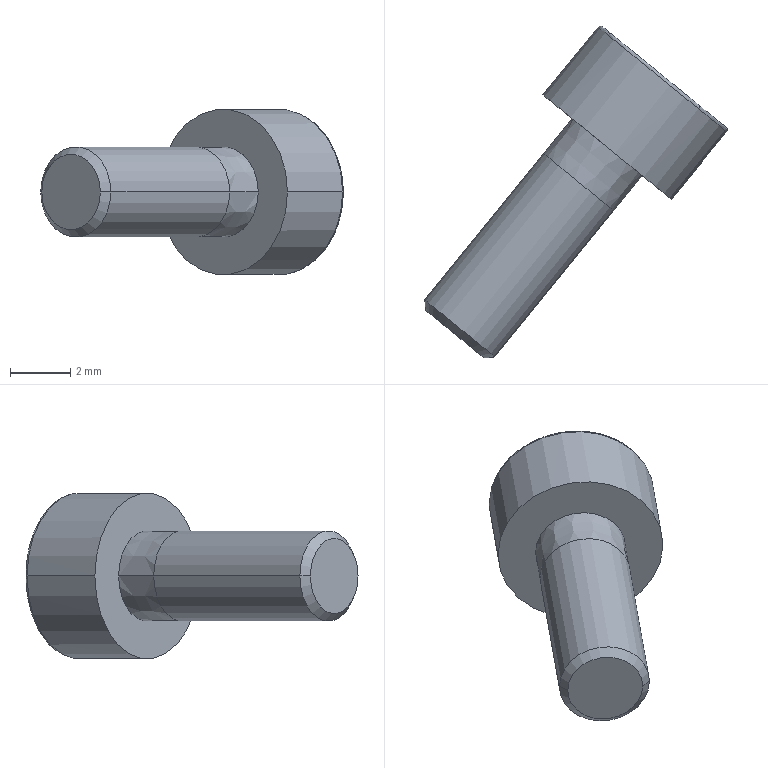Part | SolidWorks | features BaseBody 1 | 1 solid | 20 faces | box 10.039 x 11.017 x 5.5 mm | volume 120.466 mm3 | plane 10 | cylinder 4 | cone 4 | spline 2 | commonest cylinder face diameters 3 x2 5.5 x2
STEP:
#1=CARTESIAN_POINT('',(545.105,-162.622,308.898));
#2=VERTEX_POINT('',#1);
#3=CARTESIAN_POINT('',(541.772,-159.912,306.624));
#4=VERTEX_POINT('',#3);
#5=CARTESIAN_POINT('',(543.905,-161.647,306.624));
#6=DIRECTION('',(-0.6309,-0.7758,0.000000012));
#7=DIRECTION('',(0.7758,-0.6309,0.));
#8=AXIS2_PLACEMENT_3D('',#5,#6,#7);
#9=CIRCLE('',#8,2.75);
#10=EDGE_CURVE('',#2,#4,#9,.T.);
#11=ORIENTED_EDGE('',*,*,#10,.F.);
#12=CARTESIAN_POINT('',(545.124,-162.509,308.815));
#13=VERTEX_POINT('',#12);
#14=CARTESIAN_POINT('',(545.061,-162.587,308.815));
#15=DIRECTION('',(-0.6417,0.5218,0.5621));
#16=DIRECTION('',(0.4361,-0.3546,0.8271));
#17=AXIS2_PLACEMENT_3D('',#14,#15,#16);
#18=CIRCLE('',#17,0.1);
#19=EDGE_CURVE('',#2,#13,#18,.T.);
#20=ORIENTED_EDGE('',*,*,#19,.T.);
#21=CARTESIAN_POINT('',(542.813,-160.63,304.432));
#22=VERTEX_POINT('',#21);
#23=CARTESIAN_POINT('',(545.124,-162.509,308.815));
#24=CARTESIAN_POINT('',(541.723,-159.744,311.794));
#25=CARTESIAN_POINT('',(539.412,-157.864,307.411));
#26=CARTESIAN_POINT('',(542.813,-160.63,304.432));
#27=(BOUNDED_CURVE()B_SPLINE_CURVE(3,(#23,#24,#25,#26),.UNSPECIFIED.,.F.,.F.)B_SPLINE_CURVE_WITH_KNOTS((4,4),(0.,1.),.UNSPECIFIED.)CURVE()GEOMETRIC_REPRESENTATION_ITEM()RATIONAL_B_SPLINE_CURVE((1.,0.3333,0.3333,1.))REPRESENTATION_ITEM(''));
#28=EDGE_CURVE('',#13,#22,#27,.T.);
#29=ORIENTED_EDGE('',*,*,#28,.T.);
#30=CARTESIAN_POINT('',(542.706,-160.672,304.349));
#31=VERTEX_POINT('',#30);
#32=CARTESIAN_POINT('',(542.75,-160.707,304.432));
#33=DIRECTION('',(0.6417,-0.5218,-0.5621));
#34=DIRECTION('',(-0.4361,0.3546,-0.8271));
#35=AXIS2_PLACEMENT_3D('',#32,#33,#34);
#36=CIRCLE('',#35,0.1);
#37=EDGE_CURVE('',#31,#22,#36,.T.);
#38=ORIENTED_EDGE('',*,*,#37,.F.);
#39=CARTESIAN_POINT('',(543.905,-161.647,306.624));
#40=DIRECTION('',(-0.6309,-0.7758,0.000000012));
#41=DIRECTION('',(0.7758,-0.6309,0.));
#42=AXIS2_PLACEMENT_3D('',#39,#40,#41);
#43=CIRCLE('',#42,2.75);
#44=EDGE_CURVE('',#4,#31,#43,.T.);
#45=ORIENTED_EDGE('',*,*,#44,.F.);
#46=EDGE_LOOP('',(#11,#20,#29,#38,#45));
#47=FACE_OUTER_BOUND('',#46,.T.);
#48=CARTESIAN_POINT('',(545.105,-162.622,308.898));
#49=CARTESIAN_POINT('',(541.575,-159.752,311.99));
#50=CARTESIAN_POINT('',(539.177,-157.802,307.441));
#51=CARTESIAN_POINT('',(542.706,-160.672,304.349));
#52=CARTESIAN_POINT('',(545.142,-162.577,308.898));
#53=CARTESIAN_POINT('',(541.612,-159.707,311.99));
#54=CARTESIAN_POINT('',(539.214,-157.756,307.441));
#55=CARTESIAN_POINT('',(542.743,-160.627,304.349));
#56=CARTESIAN_POINT('',(545.15,-162.53,308.864));
#57=CARTESIAN_POINT('',(541.674,-159.703,311.909));
#58=CARTESIAN_POINT('',(539.311,-157.782,307.428));
#59=CARTESIAN_POINT('',(542.787,-160.609,304.383));
#60=CARTESIAN_POINT('',(545.124,-162.509,308.815));
#61=CARTESIAN_POINT('',(541.723,-159.744,311.794));
#62=CARTESIAN_POINT('',(539.412,-157.864,307.411));
#63=CARTESIAN_POINT('',(542.813,-160.63,304.432));
#64=(BOUNDED_SURFACE()B_SPLINE_SURFACE(3,3,((#48,#49,#50,#51),(#52,#53,#54,#55),(#56,#57,#58,#59),(#60,#61,#62,#63)),.UNSPECIFIED.,.F.,.F.,.F.)B_SPLINE_SURFACE_WITH_KNOTS((4,4),(4,4),(0.,1.),(0.,1.),.UNSPECIFIED.)GEOMETRIC_REPRESENTATION_ITEM()RATIONAL_B_SPLINE_SURFACE(((1.,0.3333,0.3333,1.),(0.8047,0.2682,0.2682,0.8047),(0.8047,0.2682,0.2682,0.8047),(1.,0.3333,0.3333,1.)))REPRESENTATION_ITEM('')SURFACE());
#65=ADVANCED_FACE('',(#47),#64,.T.);
#66=CARTESIAN_POINT('',(542.293,-166.007,306.624));
#67=VERTEX_POINT('',#66);
#68=CARTESIAN_POINT('',(539.966,-164.115,306.624));
#69=VERTEX_POINT('',#68);
#70=CARTESIAN_POINT('',(541.129,-165.061,306.624));
#71=DIRECTION('',(-0.6309,-0.7758,0.000000012));
#72=DIRECTION('',(0.7758,-0.6309,0.));
#73=AXIS2_PLACEMENT_3D('',#70,#71,#72);
#74=CIRCLE('',#73,1.5);
#75=EDGE_CURVE('',#67,#69,#74,.T.);
#76=ORIENTED_EDGE('',*,*,#75,.T.);
#77=CARTESIAN_POINT('',(536.022,-168.964,306.624));
#78=VERTEX_POINT('',#77);
#79=CARTESIAN_POINT('',(537.994,-166.539,306.624));
#80=DIRECTION('',(-0.6309,-0.7758,0.000000012));
#81=VECTOR('',#80,1000.);
#82=LINE('',#79,#81);
#83=EDGE_CURVE('',#69,#78,#82,.T.);
#84=ORIENTED_EDGE('',*,*,#83,.T.);
#85=CARTESIAN_POINT('',(538.35,-170.856,306.624));
#86=VERTEX_POINT('',#85);
#87=CARTESIAN_POINT('',(537.186,-169.91,306.624));
#88=DIRECTION('',(0.6309,0.7758,-0.000000012));
#89=DIRECTION('',(0.7758,-0.6309,0.));
#90=AXIS2_PLACEMENT_3D('',#87,#88,#89);
#91=CIRCLE('',#90,1.5);
#92=EDGE_CURVE('',#78,#86,#91,.T.);
#93=ORIENTED_EDGE('',*,*,#92,.T.);
#94=CARTESIAN_POINT('',(540.321,-168.432,306.624));
#95=DIRECTION('',(-0.6309,-0.7758,0.000000012));
#96=VECTOR('',#95,1000.);
#97=LINE('',#94,#96);
#98=EDGE_CURVE('',#67,#86,#97,.T.);
#99=ORIENTED_EDGE('',*,*,#98,.F.);
#100=EDGE_LOOP('',(#76,#84,#93,#99));
#101=FACE_OUTER_BOUND('',#100,.T.);
#102=CARTESIAN_POINT('',(539.158,-167.485,306.624));
#103=DIRECTION('',(-0.6309,-0.7758,0.000000012));
#104=DIRECTION('',(0.7758,-0.6309,0.));
#105=AXIS2_PLACEMENT_3D('',#102,#103,#104);
#106=CYLINDRICAL_SURFACE('',#105,1.5);
#107=ADVANCED_FACE('',(#101),#106,.T.);
#108=CARTESIAN_POINT('',(543.239,-164.843,306.624));
#109=VERTEX_POINT('',#108);
#110=CARTESIAN_POINT('',(540.913,-162.951,306.624));
#111=VERTEX_POINT('',#110);
#112=CARTESIAN_POINT('',(542.076,-163.897,306.624));
#113=DIRECTION('',(-0.6309,-0.7758,0.000000012));
#114=DIRECTION('',(0.7758,-0.6309,0.));
#115=AXIS2_PLACEMENT_3D('',#112,#113,#114);
#116=CIRCLE('',#115,1.499);
#117=EDGE_CURVE('',#109,#111,#116,.T.);
#118=ORIENTED_EDGE('',*,*,#117,.T.);
#119=CARTESIAN_POINT('',(539.966,-164.115,306.624));
#120=DIRECTION('',(-0.6313,-0.7755,0.000000012));
#121=VECTOR('',#120,1000.);
#122=LINE('',#119,#121);
#123=EDGE_CURVE('',#111,#69,#122,.T.);
#124=ORIENTED_EDGE('',*,*,#123,.T.);
#125=ORIENTED_EDGE('',*,*,#75,.F.);
#126=CARTESIAN_POINT('',(542.293,-166.007,306.624));
#127=DIRECTION('',(-0.6305,-0.7762,0.000000012));
#128=VECTOR('',#127,1000.);
#129=LINE('',#126,#128);
#130=EDGE_CURVE('',#109,#67,#129,.T.);
#131=ORIENTED_EDGE('',*,*,#130,.F.);
#132=EDGE_LOOP('',(#118,#124,#125,#131));
#133=FACE_OUTER_BOUND('',#132,.T.);
#134=CARTESIAN_POINT('',(541.129,-165.061,306.624));
#135=DIRECTION('',(-0.6309,-0.7758,0.000000012));
#136=DIRECTION('',(0.7758,-0.6309,0.));
#137=AXIS2_PLACEMENT_3D('',#134,#135,#136);
#138=CONICAL_SURFACE('',#137,1.5,0.0005);
#139=ADVANCED_FACE('',(#133),#138,.T.);
#140=CARTESIAN_POINT('',(536.058,-169.315,306.624));
#141=VERTEX_POINT('',#140);
#142=CARTESIAN_POINT('',(537.998,-170.893,306.624));
#143=VERTEX_POINT('',#142);
#144=CARTESIAN_POINT('',(537.028,-170.104,306.624));
#145=DIRECTION('',(0.6309,0.7758,-0.000000012));
#146=DIRECTION('',(-0.7758,0.6309,0.));
#147=AXIS2_PLACEMENT_3D('',#144,#145,#146);
#148=CIRCLE('',#147,1.25);
#149=EDGE_CURVE('',#141,#143,#148,.T.);
#150=ORIENTED_EDGE('',*,*,#149,.T.);
#151=CARTESIAN_POINT('',(538.35,-170.856,306.624));
#152=DIRECTION('',(0.9947,0.1025,-0.000000009));
#153=VECTOR('',#152,1000.);
#154=LINE('',#151,#153);
#155=EDGE_CURVE('',#143,#86,#154,.T.);
#156=ORIENTED_EDGE('',*,*,#155,.T.);
#157=ORIENTED_EDGE('',*,*,#92,.F.);
#158=CARTESIAN_POINT('',(536.022,-168.964,306.624));
#159=DIRECTION('',(-0.1025,0.9947,-0.000000009));
#160=VECTOR('',#159,1000.);
#161=LINE('',#158,#160);
#162=EDGE_CURVE('',#141,#78,#161,.T.);
#163=ORIENTED_EDGE('',*,*,#162,.F.);
#164=EDGE_LOOP('',(#150,#156,#157,#163));
#165=FACE_OUTER_BOUND('',#164,.T.);
#166=CARTESIAN_POINT('',(537.186,-169.91,306.624));
#167=DIRECTION('',(0.6309,0.7758,-0.000000012));
#168=DIRECTION('',(-0.7758,0.6309,0.));
#169=AXIS2_PLACEMENT_3D('',#166,#167,#168);
#170=CONICAL_SURFACE('',#169,1.5,0.7854);
#171=ADVANCED_FACE('',(#165),#170,.T.);
#172=CARTESIAN_POINT('',(546.039,-163.382,306.624));
#173=VERTEX_POINT('',#172);
#174=CARTESIAN_POINT('',(543.905,-161.647,306.624));
#175=DIRECTION('',(-0.6309,-0.7758,0.000000012));
#176=DIRECTION('',(0.7758,-0.6309,0.));
#177=AXIS2_PLACEMENT_3D('',#174,#175,#176);
#178=CIRCLE('',#177,2.75);
#179=EDGE_CURVE('',#173,#2,#178,.T.);
#180=ORIENTED_EDGE('',*,*,#179,.T.);
#181=ORIENTED_EDGE('',*,*,#10,.T.);
#182=CARTESIAN_POINT('',(539.942,-162.162,306.624));
#183=VERTEX_POINT('',#182);
#184=CARTESIAN_POINT('',(540.857,-161.037,306.624));
#185=DIRECTION('',(-0.6309,-0.7758,0.000000012));
#186=VECTOR('',#185,1000.);
#187=LINE('',#184,#186);
#188=EDGE_CURVE('',#4,#183,#187,.T.);
#189=ORIENTED_EDGE('',*,*,#188,.T.);
#190=CARTESIAN_POINT('',(544.209,-165.632,306.624));
#191=VERTEX_POINT('',#190);
#192=CARTESIAN_POINT('',(542.076,-163.897,306.624));
#193=DIRECTION('',(-0.6309,-0.7758,0.000000012));
#194=DIRECTION('',(0.7758,-0.6309,0.));
#195=AXIS2_PLACEMENT_3D('',#192,#193,#194);
#196=CIRCLE('',#195,2.75);
#197=EDGE_CURVE('',#191,#183,#196,.T.);
#198=ORIENTED_EDGE('',*,*,#197,.F.);
#199=CARTESIAN_POINT('',(545.124,-164.507,306.624));
#200=DIRECTION('',(-0.6309,-0.7758,0.000000012));
#201=VECTOR('',#200,1000.);
#202=LINE('',#199,#201);
#203=EDGE_CURVE('',#173,#191,#202,.T.);
#204=ORIENTED_EDGE('',*,*,#203,.F.);
#205=EDGE_LOOP('',(#180,#181,#189,#198,#204));
#206=FACE_OUTER_BOUND('',#205,.T.);
#207=CARTESIAN_POINT('',(542.991,-162.772,306.624));
#208=DIRECTION('',(-0.6309,-0.7758,0.000000012));
#209=DIRECTION('',(0.7758,-0.6309,0.));
#210=AXIS2_PLACEMENT_3D('',#207,#208,#209);
#211=CYLINDRICAL_SURFACE('',#210,2.75);
#212=ADVANCED_FACE('',(#206),#211,.T.);
#213=ORIENTED_EDGE('',*,*,#83,.F.);
#214=CARTESIAN_POINT('',(541.129,-165.061,306.624));
#215=DIRECTION('',(-0.6309,-0.7758,0.000000012));
#216=DIRECTION('',(0.7758,-0.6309,0.));
#217=AXIS2_PLACEMENT_3D('',#214,#215,#216);
#218=CIRCLE('',#217,1.5);
#219=EDGE_CURVE('',#69,#67,#218,.T.);
#220=ORIENTED_EDGE('',*,*,#219,.T.);
#221=ORIENTED_EDGE('',*,*,#98,.T.);
#222=CARTESIAN_POINT('',(537.186,-169.91,306.624));
#223=DIRECTION('',(0.6309,0.7758,-0.000000012));
#224=DIRECTION('',(0.7758,-0.6309,0.));
#225=AXIS2_PLACEMENT_3D('',#222,#223,#224);
#226=CIRCLE('',#225,1.5);
#227=EDGE_CURVE('',#86,#78,#226,.T.);
#228=ORIENTED_EDGE('',*,*,#227,.T.);
#229=EDGE_LOOP('',(#213,#220,#221,#228));
#230=FACE_OUTER_BOUND('',#229,.T.);
#231=CARTESIAN_POINT('',(539.158,-167.485,306.624));
#232=DIRECTION('',(-0.6309,-0.7758,0.000000012));
#233=DIRECTION('',(0.7758,-0.6309,0.));
#234=AXIS2_PLACEMENT_3D('',#231,#232,#233);
#235=CYLINDRICAL_SURFACE('',#234,1.5);
#236=ADVANCED_FACE('',(#230),#235,.T.);
#237=ORIENTED_EDGE('',*,*,#123,.F.);
#238=CARTESIAN_POINT('',(542.076,-163.897,306.624));
#239=DIRECTION('',(-0.6309,-0.7758,0.000000012));
#240=DIRECTION('',(0.7758,-0.6309,0.));
#241=AXIS2_PLACEMENT_3D('',#238,#239,#240);
#242=CIRCLE('',#241,1.499);
#243=EDGE_CURVE('',#111,#109,#242,.T.);
#244=ORIENTED_EDGE('',*,*,#243,.T.);
#245=ORIENTED_EDGE('',*,*,#130,.T.);
#246=ORIENTED_EDGE('',*,*,#219,.F.);
#247=EDGE_LOOP('',(#237,#244,#245,#246));
#248=FACE_OUTER_BOUND('',#247,.T.);
#249=CARTESIAN_POINT('',(541.129,-165.061,306.624));
#250=DIRECTION('',(-0.6309,-0.7758,0.000000012));
#251=DIRECTION('',(0.7758,-0.6309,0.));
#252=AXIS2_PLACEMENT_3D('',#249,#250,#251);
#253=CONICAL_SURFACE('',#252,1.5,0.0005);
#254=ADVANCED_FACE('',(#248),#253,.T.);
#255=ORIENTED_EDGE('',*,*,#155,.F.);
#256=CARTESIAN_POINT('',(537.028,-170.104,306.624));
#257=DIRECTION('',(0.6309,0.7758,-0.000000012));
#258=DIRECTION('',(-0.7758,0.6309,0.));
#259=AXIS2_PLACEMENT_3D('',#256,#257,#258);
#260=CIRCLE('',#259,1.25);
#261=EDGE_CURVE('',#143,#141,#260,.T.);
#262=ORIENTED_EDGE('',*,*,#261,.T.);
#263=ORIENTED_EDGE('',*,*,#162,.T.);
#264=ORIENTED_EDGE('',*,*,#227,.F.);
#265=EDGE_LOOP('',(#255,#262,#263,#264));
#266=FACE_OUTER_BOUND('',#265,.T.);
#267=CARTESIAN_POINT('',(537.186,-169.91,306.624));
#268=DIRECTION('',(0.6309,0.7758,-0.000000012));
#269=DIRECTION('',(-0.7758,0.6309,0.));
#270=AXIS2_PLACEMENT_3D('',#267,#268,#269);
#271=CONICAL_SURFACE('',#270,1.5,0.7854);
#272=ADVANCED_FACE('',(#266),#271,.T.);
#273=ORIENTED_EDGE('',*,*,#117,.F.);
#274=ORIENTED_EDGE('',*,*,#243,.F.);
#275=EDGE_LOOP('',(#273,#274));
#276=FACE_BOUND('',#275,.T.);
#277=ORIENTED_EDGE('',*,*,#197,.T.);
#278=CARTESIAN_POINT('',(542.076,-163.897,306.624));
#279=DIRECTION('',(-0.6309,-0.7758,0.000000012));
#280=DIRECTION('',(0.7758,-0.6309,0.));
#281=AXIS2_PLACEMENT_3D('',#278,#279,#280);
#282=CIRCLE('',#281,2.75);
#283=EDGE_CURVE('',#183,#191,#282,.T.);
#284=ORIENTED_EDGE('',*,*,#283,.T.);
#285=EDGE_LOOP('',(#277,#284));
#286=FACE_OUTER_BOUND('',#285,.T.);
#287=CARTESIAN_POINT('',(541.476,-163.41,305.486));
#288=DIRECTION('',(-0.6309,-0.7758,0.000000012));
#289=DIRECTION('',(0.7758,-0.6309,0.));
#290=AXIS2_PLACEMENT_3D('',#287,#288,#289);
#291=PLANE('',#290);
#292=ADVANCED_FACE('',(#276,#286),#291,.T.);
#293=ORIENTED_EDGE('',*,*,#149,.F.);
#294=ORIENTED_EDGE('',*,*,#261,.F.);
#295=EDGE_LOOP('',(#293,#294));
#296=FACE_OUTER_BOUND('',#295,.T.);
#297=CARTESIAN_POINT('',(536.756,-169.882,306.107));
#298=DIRECTION('',(-0.6309,-0.7758,0.000000012));
#299=DIRECTION('',(0.7758,-0.6309,0.));
#300=AXIS2_PLACEMENT_3D('',#297,#298,#299);
#301=PLANE('',#300);
#302=ADVANCED_FACE('',(#296),#301,.T.);
#303=ORIENTED_EDGE('',*,*,#188,.F.);
#304=ORIENTED_EDGE('',*,*,#44,.T.);
#305=CARTESIAN_POINT('',(543.905,-161.647,306.624));
#306=DIRECTION('',(-0.6309,-0.7758,0.000000012));
#307=DIRECTION('',(0.7758,-0.6309,0.));
#308=AXIS2_PLACEMENT_3D('',#305,#306,#307);
#309=CIRCLE('',#308,2.75);
#310=EDGE_CURVE('',#31,#173,#309,.T.);
#311=ORIENTED_EDGE('',*,*,#310,.T.);
#312=ORIENTED_EDGE('',*,*,#203,.T.);
#313=ORIENTED_EDGE('',*,*,#283,.F.);
#314=EDGE_LOOP('',(#303,#304,#311,#312,#313));
#315=FACE_OUTER_BOUND('',#314,.T.);
#316=CARTESIAN_POINT('',(542.991,-162.772,306.624));
#317=DIRECTION('',(-0.6309,-0.7758,0.000000012));
#318=DIRECTION('',(0.7758,-0.6309,0.));
#319=AXIS2_PLACEMENT_3D('',#316,#317,#318);
#320=CYLINDRICAL_SURFACE('',#319,2.75);
#321=ADVANCED_FACE('',(#315),#320,.T.);
#322=ORIENTED_EDGE('',*,*,#19,.F.);
#323=ORIENTED_EDGE('',*,*,#179,.F.);
#324=ORIENTED_EDGE('',*,*,#310,.F.);
#325=ORIENTED_EDGE('',*,*,#37,.T.);
#326=CARTESIAN_POINT('',(542.813,-160.63,304.432));
#327=CARTESIAN_POINT('',(546.214,-163.396,301.453));
#328=CARTESIAN_POINT('',(548.525,-165.275,305.836));
#329=CARTESIAN_POINT('',(545.124,-162.509,308.815));
#330=(BOUNDED_CURVE()B_SPLINE_CURVE(3,(#326,#327,#328,#329),.UNSPECIFIED.,.F.,.F.)B_SPLINE_CURVE_WITH_KNOTS((4,4),(0.,1.),.UNSPECIFIED.)CURVE()GEOMETRIC_REPRESENTATION_ITEM()RATIONAL_B_SPLINE_CURVE((1.,0.3333,0.3333,1.))REPRESENTATION_ITEM(''));
#331=EDGE_CURVE('',#22,#13,#330,.T.);
#332=ORIENTED_EDGE('',*,*,#331,.T.);
#333=EDGE_LOOP('',(#322,#323,#324,#325,#332));
#334=FACE_OUTER_BOUND('',#333,.T.);
#335=CARTESIAN_POINT('',(542.706,-160.672,304.349));
#336=CARTESIAN_POINT('',(546.235,-163.542,301.258));
#337=CARTESIAN_POINT('',(548.634,-165.493,305.807));
#338=CARTESIAN_POINT('',(545.105,-162.622,308.898));
#339=CARTESIAN_POINT('',(542.743,-160.627,304.349));
#340=CARTESIAN_POINT('',(546.272,-163.497,301.258));
#341=CARTESIAN_POINT('',(548.671,-165.447,305.807));
#342=CARTESIAN_POINT('',(545.142,-162.577,308.898));
#343=CARTESIAN_POINT('',(542.787,-160.609,304.383));
#344=CARTESIAN_POINT('',(546.263,-163.436,301.339));
#345=CARTESIAN_POINT('',(548.626,-165.357,305.819));
#346=CARTESIAN_POINT('',(545.15,-162.53,308.864));
#347=CARTESIAN_POINT('',(542.813,-160.63,304.432));
#348=CARTESIAN_POINT('',(546.214,-163.396,301.453));
#349=CARTESIAN_POINT('',(548.525,-165.275,305.836));
#350=CARTESIAN_POINT('',(545.124,-162.509,308.815));
#351=(BOUNDED_SURFACE()B_SPLINE_SURFACE(3,3,((#335,#336,#337,#338),(#339,#340,#341,#342),(#343,#344,#345,#346),(#347,#348,#349,#350)),.UNSPECIFIED.,.F.,.F.,.F.)B_SPLINE_SURFACE_WITH_KNOTS((4,4),(4,4),(0.,1.),(0.,1.),.UNSPECIFIED.)GEOMETRIC_REPRESENTATION_ITEM()RATIONAL_B_SPLINE_SURFACE(((1.,0.3333,0.3333,1.),(0.8047,0.2682,0.2682,0.8047),(0.8047,0.2682,0.2682,0.8047),(1.,0.3333,0.3333,1.)))REPRESENTATION_ITEM('')SURFACE());
#352=ADVANCED_FACE('',(#334),#351,.T.);
#353=ORIENTED_EDGE('',*,*,#28,.F.);
#354=ORIENTED_EDGE('',*,*,#331,.F.);
#355=EDGE_LOOP('',(#353,#354));
#356=FACE_OUTER_BOUND('',#355,.T.);
#357=CARTESIAN_POINT('',(545.085,-162.478,306.518));
#358=VERTEX_POINT('',#357);
#359=CARTESIAN_POINT('',(544.598,-162.082,307.817));
#360=VERTEX_POINT('',#359);
#361=CARTESIAN_POINT('',(545.085,-162.478,306.518));
#362=DIRECTION('',(-0.3377,0.2746,0.9003));
#363=VECTOR('',#362,1000.);
#364=LINE('',#361,#363);
#365=EDGE_CURVE('',#358,#360,#364,.T.);
#366=ORIENTED_EDGE('',*,*,#365,.T.);
#367=CARTESIAN_POINT('',(543.481,-161.173,307.923));
#368=VERTEX_POINT('',#367);
#369=CARTESIAN_POINT('',(544.598,-162.082,307.817));
#370=DIRECTION('',(-0.7738,0.6292,0.07324));
#371=VECTOR('',#370,1000.);
#372=LINE('',#369,#371);
#373=EDGE_CURVE('',#360,#368,#372,.T.);
#374=ORIENTED_EDGE('',*,*,#373,.T.);
#375=CARTESIAN_POINT('',(542.852,-160.661,306.729));
#376=VERTEX_POINT('',#375);
#377=CARTESIAN_POINT('',(543.481,-161.173,307.923));
#378=DIRECTION('',(-0.4361,0.3546,-0.8271));
#379=VECTOR('',#378,1000.);
#380=LINE('',#377,#379);
#381=EDGE_CURVE('',#368,#376,#380,.T.);
#382=ORIENTED_EDGE('',*,*,#381,.T.);
#383=CARTESIAN_POINT('',(543.339,-161.058,305.43));
#384=VERTEX_POINT('',#383);
#385=CARTESIAN_POINT('',(542.852,-160.661,306.729));
#386=DIRECTION('',(0.3377,-0.2746,-0.9003));
#387=VECTOR('',#386,1000.);
#388=LINE('',#385,#387);
#389=EDGE_CURVE('',#376,#384,#388,.T.);
#390=ORIENTED_EDGE('',*,*,#389,.T.);
#391=CARTESIAN_POINT('',(544.456,-161.966,305.324));
#392=VERTEX_POINT('',#391);
#393=CARTESIAN_POINT('',(543.339,-161.058,305.43));
#394=DIRECTION('',(0.7738,-0.6292,-0.07324));
#395=VECTOR('',#394,1000.);
#396=LINE('',#393,#395);
#397=EDGE_CURVE('',#384,#392,#396,.T.);
#398=ORIENTED_EDGE('',*,*,#397,.T.);
#399=CARTESIAN_POINT('',(544.456,-161.966,305.324));
#400=DIRECTION('',(0.4361,-0.3546,0.8271));
#401=VECTOR('',#400,1000.);
#402=LINE('',#399,#401);
#403=EDGE_CURVE('',#392,#358,#402,.T.);
#404=ORIENTED_EDGE('',*,*,#403,.T.);
#405=EDGE_LOOP('',(#366,#374,#382,#390,#398,#404));
#406=FACE_BOUND('',#405,.T.);
#407=CARTESIAN_POINT('',(543.391,-161.1,305.528));
#408=DIRECTION('',(0.6309,0.7758,-0.000000012));
#409=DIRECTION('',(-0.7758,0.6309,0.));
#410=AXIS2_PLACEMENT_3D('',#407,#408,#409);
#411=PLANE('',#410);
#412=ADVANCED_FACE('',(#356,#406),#411,.T.);
#413=CARTESIAN_POINT('',(542.661,-162.182,307.923));
#414=VERTEX_POINT('',#413);
#415=CARTESIAN_POINT('',(543.481,-161.173,307.923));
#416=DIRECTION('',(-0.6309,-0.7758,0.000000012));
#417=VECTOR('',#416,1000.);
#418=LINE('',#415,#417);
#419=EDGE_CURVE('',#368,#414,#418,.T.);
#420=ORIENTED_EDGE('',*,*,#419,.F.);
#421=ORIENTED_EDGE('',*,*,#373,.F.);
#422=CARTESIAN_POINT('',(543.778,-163.09,307.817));
#423=VERTEX_POINT('',#422);
#424=CARTESIAN_POINT('',(543.778,-163.09,307.817));
#425=DIRECTION('',(0.6309,0.7758,-0.000000012));
#426=VECTOR('',#425,1000.);
#427=LINE('',#424,#426);
#428=EDGE_CURVE('',#423,#360,#427,.T.);
#429=ORIENTED_EDGE('',*,*,#428,.F.);
#430=CARTESIAN_POINT('',(542.661,-162.182,307.923));
#431=DIRECTION('',(0.7738,-0.6292,-0.07324));
#432=VECTOR('',#431,1000.);
#433=LINE('',#430,#432);
#434=EDGE_CURVE('',#414,#423,#433,.T.);
#435=ORIENTED_EDGE('',*,*,#434,.F.);
#436=EDGE_LOOP('',(#420,#421,#429,#435));
#437=FACE_OUTER_BOUND('',#436,.T.);
#438=CARTESIAN_POINT('',(543.481,-161.173,307.923));
#439=DIRECTION('',(0.05682,-0.04621,0.9973));
#440=DIRECTION('',(0.9984,0.,-0.05688));
#441=AXIS2_PLACEMENT_3D('',#438,#439,#440);
#442=PLANE('',#441);
#443=ADVANCED_FACE('',(#437),#442,.F.);
#444=ORIENTED_EDGE('',*,*,#428,.T.);
#445=ORIENTED_EDGE('',*,*,#365,.F.);
#446=CARTESIAN_POINT('',(544.265,-163.486,306.518));
#447=VERTEX_POINT('',#446);
#448=CARTESIAN_POINT('',(545.085,-162.478,306.518));
#449=DIRECTION('',(0.6309,0.7758,0.));
#450=VECTOR('',#449,1000.);
#451=LINE('',#448,#450);
#452=EDGE_CURVE('',#447,#358,#451,.T.);
#453=ORIENTED_EDGE('',*,*,#452,.F.);
#454=CARTESIAN_POINT('',(543.778,-163.09,307.817));
#455=DIRECTION('',(0.3377,-0.2746,-0.9003));
#456=VECTOR('',#455,1000.);
#457=LINE('',#454,#456);
#458=EDGE_CURVE('',#423,#447,#457,.T.);
#459=ORIENTED_EDGE('',*,*,#458,.F.);
#460=EDGE_LOOP('',(#444,#445,#453,#459));
#461=FACE_OUTER_BOUND('',#460,.T.);
#462=CARTESIAN_POINT('',(544.598,-162.082,307.817));
#463=DIRECTION('',(0.6985,-0.568,0.4352));
#464=DIRECTION('',(0.6309,0.7758,0.));
#465=AXIS2_PLACEMENT_3D('',#462,#463,#464);
#466=PLANE('',#465);
#467=ADVANCED_FACE('',(#461),#466,.F.);
#468=ORIENTED_EDGE('',*,*,#452,.T.);
#469=ORIENTED_EDGE('',*,*,#403,.F.);
#470=CARTESIAN_POINT('',(543.636,-162.975,305.324));
#471=VERTEX_POINT('',#470);
#472=CARTESIAN_POINT('',(543.636,-162.975,305.324));
#473=DIRECTION('',(0.6309,0.7758,-0.000000012));
#474=VECTOR('',#473,1000.);
#475=LINE('',#472,#474);
#476=EDGE_CURVE('',#471,#392,#475,.T.);
#477=ORIENTED_EDGE('',*,*,#476,.F.);
#478=CARTESIAN_POINT('',(544.265,-163.486,306.518));
#479=DIRECTION('',(-0.4361,0.3546,-0.8271));
#480=VECTOR('',#479,1000.);
#481=LINE('',#478,#480);
#482=EDGE_CURVE('',#447,#471,#481,.T.);
#483=ORIENTED_EDGE('',*,*,#482,.F.);
#484=EDGE_LOOP('',(#468,#469,#477,#483));
#485=FACE_OUTER_BOUND('',#484,.T.);
#486=CARTESIAN_POINT('',(545.085,-162.478,306.518));
#487=DIRECTION('',(0.6417,-0.5218,-0.5621));
#488=DIRECTION('',(-0.6589,0.,-0.7522));
#489=AXIS2_PLACEMENT_3D('',#486,#487,#488);
#490=PLANE('',#489);
#491=ADVANCED_FACE('',(#485),#490,.F.);
#492=ORIENTED_EDGE('',*,*,#476,.T.);
#493=ORIENTED_EDGE('',*,*,#397,.F.);
#494=CARTESIAN_POINT('',(542.519,-162.066,305.43));
#495=VERTEX_POINT('',#494);
#496=CARTESIAN_POINT('',(542.519,-162.066,305.43));
#497=DIRECTION('',(0.6309,0.7758,-0.000000012));
#498=VECTOR('',#497,1000.);
#499=LINE('',#496,#498);
#500=EDGE_CURVE('',#495,#384,#499,.T.);
#501=ORIENTED_EDGE('',*,*,#500,.F.);
#502=CARTESIAN_POINT('',(543.636,-162.975,305.324));
#503=DIRECTION('',(-0.7738,0.6292,0.07324));
#504=VECTOR('',#503,1000.);
#505=LINE('',#502,#504);
#506=EDGE_CURVE('',#471,#495,#505,.T.);
#507=ORIENTED_EDGE('',*,*,#506,.F.);
#508=EDGE_LOOP('',(#492,#493,#501,#507));
#509=FACE_OUTER_BOUND('',#508,.T.);
#510=CARTESIAN_POINT('',(544.456,-161.966,305.324));
#511=DIRECTION('',(-0.05682,0.04621,-0.9973));
#512=DIRECTION('',(-0.9984,0.,0.05688));
#513=AXIS2_PLACEMENT_3D('',#510,#511,#512);
#514=PLANE('',#513);
#515=ADVANCED_FACE('',(#509),#514,.F.);
#516=ORIENTED_EDGE('',*,*,#500,.T.);
#517=ORIENTED_EDGE('',*,*,#389,.F.);
#518=CARTESIAN_POINT('',(542.031,-161.67,306.729));
#519=VERTEX_POINT('',#518);
#520=CARTESIAN_POINT('',(542.852,-160.661,306.729));
#521=DIRECTION('',(0.6309,0.7758,0.));
#522=VECTOR('',#521,1000.);
#523=LINE('',#520,#522);
#524=EDGE_CURVE('',#519,#376,#523,.T.);
#525=ORIENTED_EDGE('',*,*,#524,.F.);
#526=CARTESIAN_POINT('',(542.519,-162.066,305.43));
#527=DIRECTION('',(-0.3377,0.2746,0.9003));
#528=VECTOR('',#527,1000.);
#529=LINE('',#526,#528);
#530=EDGE_CURVE('',#495,#519,#529,.T.);
#531=ORIENTED_EDGE('',*,*,#530,.F.);
#532=EDGE_LOOP('',(#516,#517,#525,#531));
#533=FACE_OUTER_BOUND('',#532,.T.);
#534=CARTESIAN_POINT('',(543.339,-161.058,305.43));
#535=DIRECTION('',(-0.6985,0.568,-0.4352));
#536=DIRECTION('',(-0.6309,-0.7758,0.));
#537=AXIS2_PLACEMENT_3D('',#534,#535,#536);
#538=PLANE('',#537);
#539=ADVANCED_FACE('',(#533),#538,.F.);
#540=ORIENTED_EDGE('',*,*,#524,.T.);
#541=ORIENTED_EDGE('',*,*,#381,.F.);
#542=ORIENTED_EDGE('',*,*,#419,.T.);
#543=CARTESIAN_POINT('',(542.031,-161.67,306.729));
#544=DIRECTION('',(0.4361,-0.3546,0.8271));
#545=VECTOR('',#544,1000.);
#546=LINE('',#543,#545);
#547=EDGE_CURVE('',#519,#414,#546,.T.);
#548=ORIENTED_EDGE('',*,*,#547,.F.);
#549=EDGE_LOOP('',(#540,#541,#542,#548));
#550=FACE_OUTER_BOUND('',#549,.T.);
#551=CARTESIAN_POINT('',(542.852,-160.661,306.729));
#552=DIRECTION('',(-0.6417,0.5218,0.5621));
#553=DIRECTION('',(0.6589,0.,0.7522));
#554=AXIS2_PLACEMENT_3D('',#551,#552,#553);
#555=PLANE('',#554);
#556=ADVANCED_FACE('',(#550),#555,.F.);
#557=ORIENTED_EDGE('',*,*,#506,.T.);
#558=ORIENTED_EDGE('',*,*,#530,.T.);
#559=ORIENTED_EDGE('',*,*,#547,.T.);
#560=ORIENTED_EDGE('',*,*,#434,.T.);
#561=ORIENTED_EDGE('',*,*,#458,.T.);
#562=ORIENTED_EDGE('',*,*,#482,.T.);
#563=EDGE_LOOP('',(#557,#558,#559,#560,#561,#562));
#564=FACE_OUTER_BOUND('',#563,.T.);
#565=CARTESIAN_POINT('',(543.148,-162.578,306.624));
#566=DIRECTION('',(0.6309,0.7758,-0.000000012));
#567=DIRECTION('',(-0.7758,0.6309,0.));
#568=AXIS2_PLACEMENT_3D('',#565,#566,#567);
#569=PLANE('',#568);
#570=ADVANCED_FACE('',(#564),#569,.T.);
#571=CLOSED_SHELL('',(#65,#107,#139,#171,#212,#236,#254,#272,#292,#302,#321,#352,#412,#443,#467,#491,#515,#539,#556,#570));
#572=MANIFOLD_SOLID_BREP('',#571);
#573=CARTESIAN_POINT('',(0.,0.,0.));
#574=DIRECTION('',(0.,0.,1.));
#575=DIRECTION('',(1.,0.,0.));
#576=AXIS2_PLACEMENT_3D('',#573,#574,#575);
#577=(LENGTH_UNIT()NAMED_UNIT(*)SI_UNIT(.MILLI.,.METRE.));
#578=UNCERTAINTY_MEASURE_WITH_UNIT(LENGTH_MEASURE(0.00001),#577,'','');
#579=(NAMED_UNIT(*)PLANE_ANGLE_UNIT()SI_UNIT($,.RADIAN.));
#580=(NAMED_UNIT(*)SI_UNIT($,.STERADIAN.)SOLID_ANGLE_UNIT());
#581=(GEOMETRIC_REPRESENTATION_CONTEXT(3)GLOBAL_UNCERTAINTY_ASSIGNED_CONTEXT((#578))GLOBAL_UNIT_ASSIGNED_CONTEXT((#577,#579,#580))REPRESENTATION_CONTEXT('',''));
#582=ADVANCED_BREP_SHAPE_REPRESENTATION('',(#572,#576),#581);